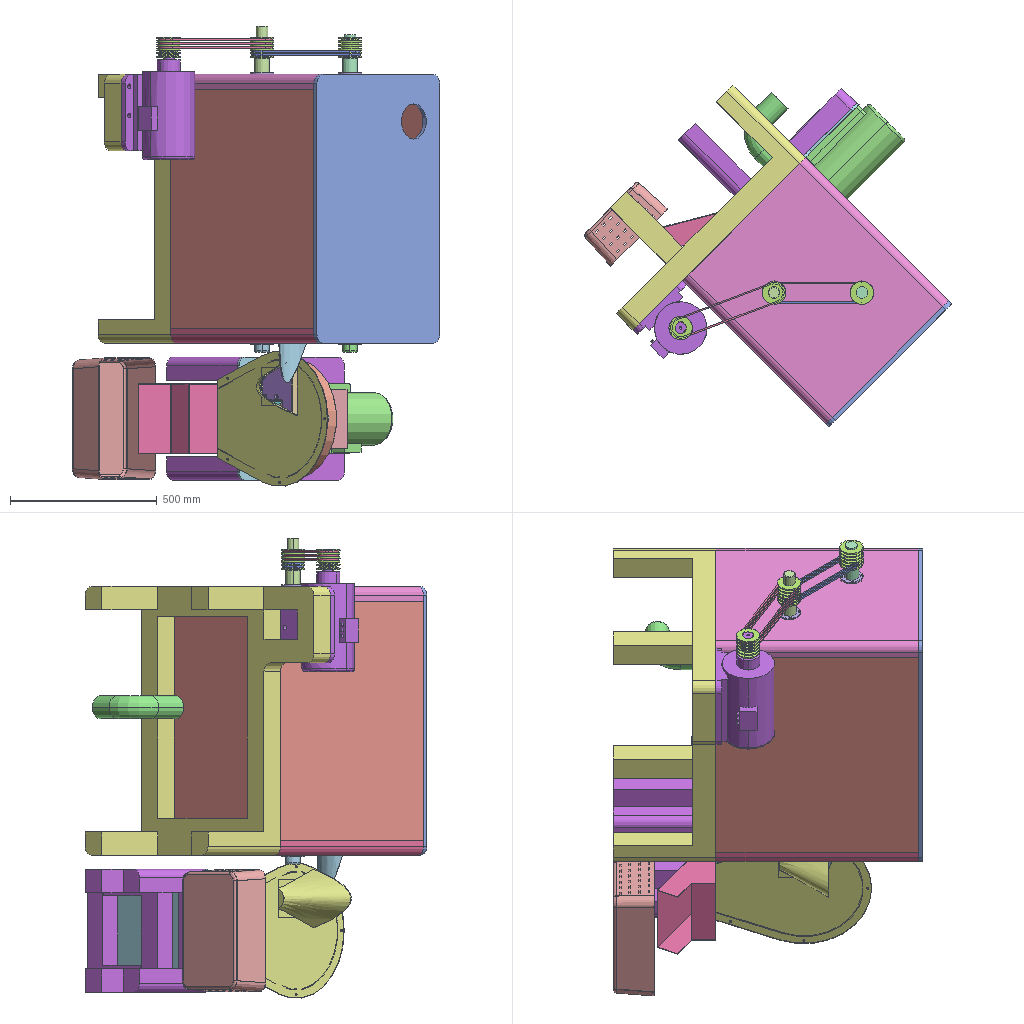Assembly | SolidWorks | 462 different items | 999 placed | box 1253 x 1165 x 1569 mm
Parts list (item | name | quantity | parent item | size | volume | features):
1 | (subassembly) | x1 | in 13 | 390 x 75.007 x 390 mm | 1088681 mm3 | features AEMSimFeature 1
2 | (subassembly) | x1 | in 15 | 456 x 70 x 529.065 mm | 279476 mm3 | features AEMSimFeature 1
3 | (subassembly) | x1 | in 15 | 462 x 531 x 183 mm | 626105 mm3 | features AEMSimFeature 1
4 | (subassembly) | x1 | in 6 | 462 x 872.289 x 730.81 mm | 20879120 mm3 | features AEMSimFeature 1
5 | (subassembly) | x1 | - | 839.689 x 835.894 x 1384 mm | 47233024 mm3 | features AEMSimFeature 1
6 | (subassembly) | x1 | - | - | 106824428 mm3 | features AEMSimFeature 1
7 | (subassembly) | x2 | in 6 | 787.42 x 340 x 340 mm | 9693964 mm3 | features AEMSimFeature 1
8 | (subassembly) | x4 | in 6 | 68 x 19 x 68 mm | 29174 mm3 | features AEMSimFeature 1
9 | (subassembly) | x4 | in 10 | 68 x 68 x 19 mm | 27865 mm3 | features AEMSimFeature 1
10 | (subassembly) | x4 | in 8 | 68 x 19 x 68 mm | 29174 mm3 | features AEMSimFeature 1
11 | (subassembly) | x1 | in 15 | 14 x 62 x 62 mm | 20908 mm3 | features AEMSimFeature 1
12 | (subassembly) | x1 | in 15 | 14 x 62 x 62 mm | 20908 mm3 | features AEMSimFeature 1
13 | (subassembly) | x1 | in 15 | 390 x 210.007 x 390 mm | 3767306 mm3 | features AEMSimFeature 1
14 | (subassembly) | x1 | in 16 | 462 x 451 x 532.065 mm | 5080659 mm3 | features AEMSimFeature 1
15 | (subassembly) | x1 | in 14 | 462 x 532.065 x 451 mm | 5080659 mm3 | features AEMSimFeature 1
16 | (subassembly) | x1 | in 4 | 462 x 451 x 532.065 mm | 5080659 mm3 | features AEMSimFeature 1
17 | (subassembly) | x1 | in 1 | 72 x 14 x 72 mm | 4934 mm3 | features AEMSimFeature 1
18 | - | x2 | in 7 | 10 x 10 x 120 mm | 9425 mm3 | -
19 | - | x2 | in 7 | 10 x 78.624 x 102.96 mm | 9425 mm3 | -
20 | - | x2 | in 7 | 10 x 78.624 x 102.96 mm | 9425 mm3 | -
21 | - | x2 | in 7 | 10 x 102.96 x 78.624 mm | 9425 mm3 | -
22 | - | x2 | in 7 | 10 x 78.624 x 102.96 mm | 9425 mm3 | -
23 | - | x2 | in 7 | 10 x 46.593 x 117.217 mm | 9425 mm3 | -
24 | - | x2 | in 7 | 10 x 102.96 x 78.624 mm | 9425 mm3 | -
25 | - | x2 | in 7 | 10 x 78.624 x 102.96 mm | 9425 mm3 | -
26 | - | x2 | in 7 | 10 x 102.96 x 78.624 mm | 9425 mm3 | -
27 | - | x2 | in 7 | 10 x 46.593 x 117.217 mm | 9425 mm3 | -
28 | - | x2 | in 7 | 10 x 78.624 x 102.96 mm | 9425 mm3 | -
29 | - | x2 | in 7 | 10 x 10 x 120 mm | 9425 mm3 | -
30 | - | x2 | in 7 | 10 x 10 x 120 mm | 9425 mm3 | -
31 | - | x2 | in 7 | 10 x 46.593 x 117.217 mm | 9425 mm3 | -
32 | - | x2 | in 7 | 10 x 10 x 120 mm | 9425 mm3 | -
33 | - | x2 | in 7 | 10 x 78.624 x 102.96 mm | 9425 mm3 | -
34 | - | x2 | in 7 | 10 x 102.96 x 78.624 mm | 9425 mm3 | -
35 | - | x2 | in 7 | 10 x 120 x 10 mm | 9425 mm3 | -
36 | - | x2 | in 7 | 10 x 10 x 120 mm | 9425 mm3 | -
37 | - | x2 | in 7 | 10 x 10 x 120 mm | 9425 mm3 | -
38 | - | x2 | in 7 | 10 x 102.96 x 78.624 mm | 9425 mm3 | -
39 | - | x2 | in 7 | 10 x 120 x 10 mm | 9425 mm3 | -
40 | - | x2 | in 7 | 10 x 78.624 x 102.96 mm | 9425 mm3 | -
41 | - | x2 | in 7 | 10 x 117.217 x 46.593 mm | 9425 mm3 | -
42 | - | x2 | in 7 | 10 x 102.96 x 78.624 mm | 9425 mm3 | -
43 | - | x2 | in 7 | 10 x 117.217 x 46.593 mm | 9425 mm3 | -
44 | - | x2 | in 7 | 10 x 78.624 x 102.96 mm | 9425 mm3 | -
45 | - | x2 | in 7 | 10 x 78.624 x 102.96 mm | 9425 mm3 | -
46 | - | x2 | in 7 | 10 x 117.217 x 46.593 mm | 9425 mm3 | -
47 | - | x2 | in 7 | 10 x 117.217 x 46.593 mm | 9425 mm3 | -
48 | - | x2 | in 7 | 10 x 46.593 x 117.217 mm | 9425 mm3 | -
49 | - | x2 | in 7 | 10 x 46.593 x 117.217 mm | 9425 mm3 | -
50 | - | x2 | in 7 | 10 x 117.217 x 46.593 mm | 9425 mm3 | -
51 | - | x2 | in 7 | 10 x 46.593 x 117.217 mm | 9425 mm3 | -
52 | - | x2 | in 7 | 10 x 102.96 x 78.624 mm | 9425 mm3 | -
53 | - | x2 | in 7 | 10 x 10 x 120 mm | 9425 mm3 | -
54 | - | x2 | in 7 | 10 x 117.217 x 46.593 mm | 9425 mm3 | -
55 | - | x2 | in 7 | 10 x 117.217 x 46.593 mm | 9425 mm3 | -
56 | - | x2 | in 7 | 10 x 46.593 x 117.217 mm | 9425 mm3 | -
57 | - | x2 | in 7 | 10 x 46.593 x 117.217 mm | 9425 mm3 | -
58 | - | x2 | in 7 | 10 x 102.96 x 78.624 mm | 9425 mm3 | -
59 | - | x2 | in 7 | 10 x 102.96 x 78.624 mm | 9425 mm3 | -
60 | - | x2 | in 7 | 10 x 78.624 x 102.96 mm | 9425 mm3 | -
61 | - | x2 | in 7 | 10 x 120 x 10 mm | 9425 mm3 | -
62 | - | x2 | in 7 | 10 x 46.593 x 117.217 mm | 9425 mm3 | -
63 | - | x2 | in 7 | 10 x 117.217 x 46.593 mm | 9425 mm3 | -
64 | - | x2 | in 7 | 10 x 120 x 10 mm | 9425 mm3 | -
65 | - | x2 | in 7 | 10 x 78.624 x 102.96 mm | 9425 mm3 | -
66 | - | x2 | in 7 | 10 x 10 x 120 mm | 9425 mm3 | -
67 | - | x2 | in 7 | 10 x 120 x 10 mm | 9425 mm3 | -
68 | - | x2 | in 7 | 10 x 117.217 x 46.593 mm | 9425 mm3 | -
69 | - | x2 | in 7 | 10 x 117.217 x 46.593 mm | 9425 mm3 | -
70 | - | x2 | in 7 | 10 x 120 x 10 mm | 9425 mm3 | -
71 | - | x2 | in 7 | 10 x 117.217 x 46.593 mm | 9425 mm3 | -
72 | - | x2 | in 7 | 10 x 117.217 x 46.593 mm | 9425 mm3 | -
73 | - | x2 | in 7 | 10 x 10 x 120 mm | 9425 mm3 | -
74 | - | x2 | in 7 | 10 x 78.624 x 102.96 mm | 9425 mm3 | -
75 | - | x2 | in 7 | 10 x 120 x 10 mm | 9425 mm3 | -
76 | - | x2 | in 7 | 10 x 102.96 x 78.624 mm | 9425 mm3 | -
77 | - | x2 | in 7 | 10 x 46.593 x 117.217 mm | 9425 mm3 | -
78 | - | x2 | in 7 | 10 x 120 x 10 mm | 9425 mm3 | -
79 | - | x2 | in 7 | 10 x 102.96 x 78.624 mm | 9425 mm3 | -
80 | - | x2 | in 7 | 10 x 117.217 x 46.593 mm | 9425 mm3 | -
81 | - | x2 | in 7 | 10 x 117.217 x 46.593 mm | 9425 mm3 | -
82 | - | x2 | in 7 | 10 x 46.593 x 117.217 mm | 9425 mm3 | -
83 | - | x2 | in 7 | 10 x 120 x 10 mm | 9425 mm3 | -
84 | - | x2 | in 7 | 10 x 117.217 x 46.593 mm | 9425 mm3 | -
85 | - | x2 | in 7 | 10 x 117.217 x 46.593 mm | 9425 mm3 | -
86 | - | x2 | in 7 | 10 x 78.624 x 102.96 mm | 9425 mm3 | -
87 | - | x2 | in 7 | 10 x 46.593 x 117.217 mm | 9425 mm3 | -
88 | - | x2 | in 7 | 10 x 46.593 x 117.217 mm | 9425 mm3 | -
89 | - | x2 | in 7 | 10 x 10 x 120 mm | 9425 mm3 | -
90 | - | x2 | in 7 | 10 x 78.624 x 102.96 mm | 9425 mm3 | -
91 | - | x2 | in 7 | 10 x 78.624 x 102.96 mm | 9425 mm3 | -
92 | - | x2 | in 7 | 10 x 102.96 x 78.624 mm | 9425 mm3 | -
93 | - | x2 | in 7 | 10 x 102.96 x 78.624 mm | 9425 mm3 | -
94 | - | x2 | in 7 | 10 x 120 x 10 mm | 9425 mm3 | -
95 | - | x2 | in 7 | 10 x 102.96 x 78.624 mm | 9425 mm3 | -
96 | - | x2 | in 7 | 10 x 78.624 x 102.96 mm | 9425 mm3 | -
97 | - | x2 | in 7 | 10 x 102.96 x 78.624 mm | 9425 mm3 | -
98 | - | x2 | in 7 | 10 x 102.96 x 78.624 mm | 9425 mm3 | -
99 | - | x2 | in 7 | 10 x 117.217 x 46.593 mm | 9425 mm3 | -
100 | - | x2 | in 7 | 10 x 10 x 120 mm | 9425 mm3 | -
101 | - | x2 | in 7 | 10 x 117.217 x 46.593 mm | 9425 mm3 | -
102 | - | x2 | in 7 | 10 x 78.624 x 102.96 mm | 9425 mm3 | -
103 | - | x2 | in 7 | 10 x 78.624 x 102.96 mm | 9425 mm3 | -
104 | - | x2 | in 7 | 10 x 10 x 120 mm | 9425 mm3 | -
105 | - | x2 | in 7 | 10 x 117.217 x 46.593 mm | 9425 mm3 | -
106 | - | x2 | in 7 | 10 x 46.593 x 117.217 mm | 9425 mm3 | -
107 | - | x2 | in 7 | 10 x 46.593 x 117.217 mm | 9425 mm3 | -
108 | - | x2 | in 7 | 10 x 102.96 x 78.624 mm | 9425 mm3 | -
109 | - | x2 | in 7 | 10 x 10 x 120 mm | 9425 mm3 | -
110 | - | x2 | in 7 | 10 x 78.624 x 102.96 mm | 9425 mm3 | -
111 | - | x2 | in 7 | 10 x 102.96 x 78.624 mm | 9425 mm3 | -
112 | - | x2 | in 7 | 10 x 46.593 x 117.217 mm | 9425 mm3 | -
113 | - | x2 | in 7 | 10 x 78.624 x 102.96 mm | 9425 mm3 | -
114 | - | x2 | in 7 | 10 x 46.593 x 117.217 mm | 9425 mm3 | -
115 | - | x2 | in 7 | 10 x 46.593 x 117.217 mm | 9425 mm3 | -
116 | - | x2 | in 7 | 10 x 102.96 x 78.624 mm | 9425 mm3 | -
117 | - | x2 | in 7 | 10 x 117.217 x 46.593 mm | 9425 mm3 | -
118 | - | x2 | in 7 | 10 x 78.624 x 102.96 mm | 9425 mm3 | -
119 | - | x2 | in 7 | 10 x 117.217 x 46.593 mm | 9425 mm3 | -
120 | - | x2 | in 7 | 10 x 78.624 x 102.96 mm | 9425 mm3 | -
121 | - | x2 | in 7 | 10 x 120 x 10 mm | 9425 mm3 | -
122 | - | x2 | in 7 | 10 x 78.624 x 102.96 mm | 9425 mm3 | -
123 | - | x2 | in 7 | 10 x 10 x 120 mm | 9425 mm3 | -
124 | - | x2 | in 7 | 10 x 117.217 x 46.593 mm | 9425 mm3 | -
125 | - | x2 | in 7 | 10 x 102.96 x 78.624 mm | 9425 mm3 | -
126 | - | x2 | in 7 | 10 x 102.96 x 78.624 mm | 9425 mm3 | -
127 | - | x2 | in 7 | 10 x 46.593 x 117.217 mm | 9425 mm3 | -
128 | - | x4 | in 9 | 49 x 49 x 19 mm | 11442 mm3 | -
129 | - | x2 | in 7 | 10 x 46.593 x 117.217 mm | 9425 mm3 | -
130 | - | x2 | in 7 | 10 x 102.96 x 78.624 mm | 9425 mm3 | -
131 | - | x2 | in 7 | 10 x 120 x 10 mm | 9425 mm3 | -
132 | - | x2 | in 7 | 10 x 46.593 x 117.217 mm | 9425 mm3 | -
133 | - | x2 | in 7 | 10 x 46.593 x 117.217 mm | 9425 mm3 | -
134 | - | x2 | in 7 | 10 x 46.593 x 117.217 mm | 9425 mm3 | -
135 | - | x2 | in 7 | 10 x 46.593 x 117.217 mm | 9425 mm3 | -
136 | - | x2 | in 7 | 10 x 102.96 x 78.624 mm | 9425 mm3 | -
137 | - | x2 | in 7 | 10 x 102.96 x 78.624 mm | 9425 mm3 | -
138 | - | x2 | in 7 | 10 x 46.593 x 117.217 mm | 9425 mm3 | -
139 | - | x2 | in 7 | 10 x 102.96 x 78.624 mm | 9425 mm3 | -
140 | - | x2 | in 7 | 10 x 102.96 x 78.624 mm | 9425 mm3 | -
141 | - | x2 | in 7 | 10 x 78.624 x 102.96 mm | 9425 mm3 | -
142 | - | x2 | in 7 | 10 x 78.624 x 102.96 mm | 9425 mm3 | -
143 | - | x2 | in 7 | 10 x 46.593 x 117.217 mm | 9425 mm3 | -
144 | - | x2 | in 7 | 10 x 78.624 x 102.96 mm | 9425 mm3 | -
145 | - | x2 | in 7 | 10 x 117.217 x 46.593 mm | 9425 mm3 | -
146 | - | x2 | in 7 | 10 x 78.624 x 102.96 mm | 9425 mm3 | -
147 | - | x2 | in 7 | 10 x 117.217 x 46.593 mm | 9425 mm3 | -
148 | - | x2 | in 7 | 10 x 46.593 x 117.217 mm | 9425 mm3 | -
149 | - | x2 | in 7 | 10 x 46.593 x 117.217 mm | 9425 mm3 | -
150 | - | x2 | in 7 | 10 x 117.217 x 46.593 mm | 9425 mm3 | -
151 | - | x2 | in 7 | 10 x 78.624 x 102.96 mm | 9425 mm3 | -
152 | - | x2 | in 7 | 10 x 10 x 120 mm | 9425 mm3 | -
153 | - | x2 | in 7 | 10 x 46.593 x 117.217 mm | 9425 mm3 | -
154 | - | x2 | in 7 | 10 x 78.624 x 102.96 mm | 9425 mm3 | -
155 | - | x2 | in 7 | 10 x 78.624 x 102.96 mm | 9425 mm3 | -
156 | - | x2 | in 7 | 10 x 102.96 x 78.624 mm | 9425 mm3 | -
157 | - | x2 | in 7 | 10 x 78.624 x 102.96 mm | 9425 mm3 | -
158 | - | x2 | in 7 | 10 x 102.96 x 78.624 mm | 9425 mm3 | -
159 | - | x2 | in 7 | 10 x 46.593 x 117.217 mm | 9425 mm3 | -
160 | - | x2 | in 7 | 10 x 102.96 x 78.624 mm | 9425 mm3 | -
161 | - | x2 | in 7 | 10 x 102.96 x 78.624 mm | 9425 mm3 | -
162 | - | x2 | in 7 | 10 x 117.217 x 46.593 mm | 9425 mm3 | -
163 | - | x2 | in 7 | 10 x 10 x 120 mm | 9425 mm3 | -
164 | - | x2 | in 7 | 10 x 46.593 x 117.217 mm | 9425 mm3 | -
165 | - | x2 | in 7 | 10 x 78.624 x 102.96 mm | 9425 mm3 | -
166 | - | x2 | in 7 | 10 x 117.217 x 46.593 mm | 9425 mm3 | -
167 | - | x2 | in 7 | 10 x 117.217 x 46.593 mm | 9425 mm3 | -
168 | - | x2 | in 7 | 10 x 46.593 x 117.217 mm | 9425 mm3 | -
169 | - | x2 | in 7 | 10 x 78.624 x 102.96 mm | 9425 mm3 | -
170 | - | x2 | in 7 | 10 x 46.593 x 117.217 mm | 9425 mm3 | -
171 | - | x2 | in 7 | 10 x 117.217 x 46.593 mm | 9425 mm3 | -
172 | - | x2 | in 7 | 10 x 117.217 x 46.593 mm | 9425 mm3 | -
173 | - | x2 | in 7 | 10 x 78.624 x 102.96 mm | 9425 mm3 | -
174 | - | x2 | in 7 | 10 x 46.593 x 117.217 mm | 9425 mm3 | -
175 | - | x2 | in 7 | 10 x 120 x 10 mm | 9425 mm3 | -
176 | - | x2 | in 7 | 10 x 78.624 x 102.96 mm | 9425 mm3 | -
177 | - | x2 | in 7 | 10 x 102.96 x 78.624 mm | 9425 mm3 | -
178 | - | x2 | in 7 | 10 x 78.624 x 102.96 mm | 9425 mm3 | -
179 | - | x2 | in 7 | 10 x 120 x 10 mm | 9425 mm3 | -
180 | - | x2 | in 7 | 10 x 102.96 x 78.624 mm | 9425 mm3 | -
181 | - | x2 | in 7 | 10 x 117.217 x 46.593 mm | 9425 mm3 | -
182 | - | x2 | in 7 | 10 x 117.217 x 46.593 mm | 9425 mm3 | -
183 | - | x2 | in 7 | 10 x 120 x 10 mm | 9425 mm3 | -
184 | - | x2 | in 7 | 10 x 102.96 x 78.624 mm | 9425 mm3 | -
185 | - | x2 | in 7 | 10 x 102.96 x 78.624 mm | 9425 mm3 | -
186 | - | x2 | in 7 | 10 x 78.624 x 102.96 mm | 9425 mm3 | -
187 | - | x2 | in 7 | 10 x 120 x 10 mm | 9425 mm3 | -
188 | - | x2 | in 7 | 10 x 117.217 x 46.593 mm | 9425 mm3 | -
189 | - | x2 | in 7 | 10 x 117.217 x 46.593 mm | 9425 mm3 | -
190 | - | x2 | in 7 | 10 x 46.593 x 117.217 mm | 9425 mm3 | -
191 | - | x2 | in 7 | 10 x 78.624 x 102.96 mm | 9425 mm3 | -
192 | - | x2 | in 7 | 10 x 102.96 x 78.624 mm | 9425 mm3 | -
193 | - | x2 | in 7 | 10 x 102.96 x 78.624 mm | 9425 mm3 | -
194 | - | x2 | in 7 | 10 x 46.593 x 117.217 mm | 9425 mm3 | -
195 | - | x2 | in 7 | 10 x 117.217 x 46.593 mm | 9425 mm3 | -
196 | - | x2 | in 7 | 10 x 78.624 x 102.96 mm | 9425 mm3 | -
197 | - | x2 | in 7 | 10 x 120 x 10 mm | 9425 mm3 | -
198 | - | x2 | in 7 | 10 x 117.217 x 46.593 mm | 9425 mm3 | -
199 | - | x2 | in 7 | 10 x 78.624 x 102.96 mm | 9425 mm3 | -
200 | - | x2 | in 7 | 10 x 46.593 x 117.217 mm | 9425 mm3 | -
201 | - | x2 | in 7 | 10 x 46.593 x 117.217 mm | 9425 mm3 | -
202 | - | x2 | in 7 | 10 x 10 x 120 mm | 9425 mm3 | -
203 | - | x2 | in 7 | 10 x 46.593 x 117.217 mm | 9425 mm3 | -
204 | - | x2 | in 7 | 10 x 102.96 x 78.624 mm | 9425 mm3 | -
205 | - | x2 | in 7 | 10 x 78.624 x 102.96 mm | 9425 mm3 | -
206 | - | x2 | in 7 | 10 x 102.96 x 78.624 mm | 9425 mm3 | -
207 | - | x2 | in 7 | 10 x 78.624 x 102.96 mm | 9425 mm3 | -
208 | - | x2 | in 7 | 10 x 46.593 x 117.217 mm | 9425 mm3 | -
209 | - | x2 | in 7 | 10 x 78.624 x 102.96 mm | 9425 mm3 | -
210 | - | x2 | in 7 | 10 x 46.593 x 117.217 mm | 9425 mm3 | -
211 | - | x2 | in 7 | 10 x 78.624 x 102.96 mm | 9425 mm3 | -
212 | - | x2 | in 7 | 10 x 46.593 x 117.217 mm | 9425 mm3 | -
213 | - | x2 | in 7 | 10 x 10 x 120 mm | 9425 mm3 | -
214 | - | x2 | in 7 | 10 x 117.217 x 46.593 mm | 9425 mm3 | -
215 | - | x2 | in 7 | 10 x 78.624 x 102.96 mm | 9425 mm3 | -
216 | - | x2 | in 7 | 10 x 117.217 x 46.593 mm | 9425 mm3 | -
217 | - | x2 | in 7 | 10 x 10 x 120 mm | 9425 mm3 | -
218 | - | x2 | in 7 | 10 x 117.217 x 46.593 mm | 9425 mm3 | -
219 | - | x2 | in 7 | 10 x 120 x 10 mm | 9425 mm3 | -
220 | - | x2 | in 7 | 10 x 46.593 x 117.217 mm | 9425 mm3 | -
221 | - | x2 | in 7 | 10 x 46.593 x 117.217 mm | 9425 mm3 | -
222 | - | x2 | in 7 | 10 x 117.217 x 46.593 mm | 9425 mm3 | -
223 | - | x2 | in 7 | 10 x 120 x 10 mm | 9425 mm3 | -
224 | - | x2 | in 7 | 10 x 78.624 x 102.96 mm | 9425 mm3 | -
225 | - | x2 | in 7 | 10 x 78.624 x 102.96 mm | 9425 mm3 | -
226 | - | x2 | in 7 | 10 x 46.593 x 117.217 mm | 9425 mm3 | -
227 | - | x2 | in 7 | 10 x 46.593 x 117.217 mm | 9425 mm3 | -
228 | - | x2 | in 7 | 10 x 10 x 120 mm | 9425 mm3 | -
229 | - | x2 | in 7 | 10 x 10 x 120 mm | 9425 mm3 | -
230 | - | x2 | in 7 | 10 x 10 x 120 mm | 9425 mm3 | -
231 | - | x2 | in 7 | 10 x 46.593 x 117.217 mm | 9425 mm3 | -
232 | - | x2 | in 7 | 10 x 102.96 x 78.624 mm | 9425 mm3 | -
233 | - | x2 | in 7 | 10 x 46.593 x 117.217 mm | 9425 mm3 | -
234 | - | x2 | in 7 | 10 x 117.217 x 46.593 mm | 9425 mm3 | -
235 | - | x2 | in 7 | 10 x 120 x 10 mm | 9425 mm3 | -
236 | - | x2 | in 7 | 10 x 117.217 x 46.593 mm | 9425 mm3 | -
237 | - | x2 | in 7 | 10 x 117.217 x 46.593 mm | 9425 mm3 | -
238 | - | x2 | in 7 | 10 x 117.217 x 46.593 mm | 9425 mm3 | -
239 | - | x4 | in 9 | 68 x 68 x 19 mm | 16423 mm3 | -
240 | - | x2 | in 7 | 10 x 78.624 x 102.96 mm | 9425 mm3 | -
241 | - | x2 | in 7 | 10 x 78.624 x 102.96 mm | 9425 mm3 | -
242 | - | x2 | in 7 | 10 x 120 x 10 mm | 9425 mm3 | -
243 | - | x2 | in 7 | 10 x 78.624 x 102.96 mm | 9425 mm3 | -
244 | - | x2 | in 7 | 10 x 78.624 x 102.96 mm | 9425 mm3 | -
245 | - | x2 | in 7 | 10 x 102.96 x 78.624 mm | 9425 mm3 | -
246 | - | x2 | in 7 | 10 x 102.96 x 78.624 mm | 9425 mm3 | -
247 | - | x2 | in 7 | 10 x 46.593 x 117.217 mm | 9425 mm3 | -
248 | - | x2 | in 7 | 10 x 78.624 x 102.96 mm | 9425 mm3 | -
249 | - | x2 | in 7 | 10 x 120 x 10 mm | 9425 mm3 | -
250 | - | x2 | in 7 | 10 x 102.96 x 78.624 mm | 9425 mm3 | -
251 | - | x2 | in 7 | 10 x 10 x 120 mm | 9425 mm3 | -
252 | - | x2 | in 7 | 10 x 102.96 x 78.624 mm | 9425 mm3 | -
253 | - | x2 | in 7 | 10 x 120 x 10 mm | 9425 mm3 | -
254 | - | x2 | in 7 | 10 x 120 x 10 mm | 9425 mm3 | -
255 | - | x2 | in 7 | 10 x 46.593 x 117.217 mm | 9425 mm3 | -
256 | - | x2 | in 7 | 10 x 10 x 120 mm | 9425 mm3 | -
257 | - | x2 | in 7 | 10 x 10 x 120 mm | 9425 mm3 | -
258 | - | x2 | in 7 | 10 x 46.593 x 117.217 mm | 9425 mm3 | -
259 | - | x2 | in 7 | 10 x 102.96 x 78.624 mm | 9425 mm3 | -
260 | - | x2 | in 7 | 10 x 10 x 120 mm | 9425 mm3 | -
261 | - | x2 | in 7 | 10 x 120 x 10 mm | 9425 mm3 | -
262 | - | x2 | in 7 | 10 x 120 x 10 mm | 9425 mm3 | -
263 | - | x2 | in 7 | 10 x 117.217 x 46.593 mm | 9425 mm3 | -
264 | - | x2 | in 7 | 10 x 117.217 x 46.593 mm | 9425 mm3 | -
265 | - | x2 | in 7 | 10 x 46.593 x 117.217 mm | 9425 mm3 | -
266 | - | x2 | in 7 | 10 x 46.593 x 117.217 mm | 9425 mm3 | -
267 | - | x2 | in 7 | 10 x 117.217 x 46.593 mm | 9425 mm3 | -
268 | - | x2 | in 7 | 10 x 117.217 x 46.593 mm | 9425 mm3 | -
269 | - | x2 | in 7 | 10 x 102.96 x 78.624 mm | 9425 mm3 | -
270 | - | x2 | in 7 | 10 x 46.593 x 117.217 mm | 9425 mm3 | -
271 | - | x2 | in 7 | 10 x 102.96 x 78.624 mm | 9425 mm3 | -
272 | - | x2 | in 7 | 10 x 10 x 120 mm | 9425 mm3 | -
273 | - | x2 | in 7 | 10 x 120 x 10 mm | 9425 mm3 | -
274 | - | x2 | in 7 | 10 x 78.624 x 102.96 mm | 9425 mm3 | -
275 | - | x2 | in 7 | 10 x 10 x 120 mm | 9425 mm3 | -
276 | - | x2 | in 7 | 10 x 10 x 120 mm | 9425 mm3 | -
277 | - | x2 | in 7 | 10 x 102.96 x 78.624 mm | 9425 mm3 | -
278 | - | x2 | in 7 | 10 x 78.624 x 102.96 mm | 9425 mm3 | -
279 | - | x2 | in 7 | 10 x 102.96 x 78.624 mm | 9425 mm3 | -
280 | - | x2 | in 7 | 10 x 78.624 x 102.96 mm | 9425 mm3 | -
281 | - | x2 | in 7 | 10 x 117.217 x 46.593 mm | 9425 mm3 | -
282 | - | x2 | in 7 | 10 x 78.624 x 102.96 mm | 9425 mm3 | -
283 | - | x2 | in 7 | 10 x 120 x 10 mm | 9425 mm3 | -
284 | - | x2 | in 7 | 10 x 102.96 x 78.624 mm | 9425 mm3 | -
285 | - | x2 | in 7 | 10 x 102.96 x 78.624 mm | 9425 mm3 | -
286 | - | x2 | in 7 | 10 x 78.624 x 102.96 mm | 9425 mm3 | -
287 | - | x2 | in 7 | 10 x 102.96 x 78.624 mm | 9425 mm3 | -
288 | - | x2 | in 7 | 10 x 102.96 x 78.624 mm | 9425 mm3 | -
289 | - | x2 | in 7 | 10 x 102.96 x 78.624 mm | 9425 mm3 | -
290 | - | x2 | in 7 | 10 x 120 x 10 mm | 9425 mm3 | -
291 | - | x2 | in 7 | 10 x 120 x 10 mm | 9425 mm3 | -
292 | - | x2 | in 7 | 10 x 46.593 x 117.217 mm | 9425 mm3 | -
293 | - | x2 | in 7 | 10 x 78.624 x 102.96 mm | 9425 mm3 | -
294 | - | x2 | in 7 | 10 x 78.624 x 102.96 mm | 9425 mm3 | -
295 | - | x2 | in 7 | 10 x 102.96 x 78.624 mm | 9425 mm3 | -
296 | - | x2 | in 7 | 10 x 10 x 120 mm | 9425 mm3 | -
297 | - | x2 | in 7 | 10 x 102.96 x 78.624 mm | 9425 mm3 | -
298 | - | x2 | in 7 | 10 x 46.593 x 117.217 mm | 9425 mm3 | -
299 | - | x2 | in 7 | 10 x 46.593 x 117.217 mm | 9425 mm3 | -
300 | - | x2 | in 7 | 10 x 117.217 x 46.593 mm | 9425 mm3 | -
301 | - | x2 | in 7 | 10 x 10 x 120 mm | 9425 mm3 | -
302 | - | x2 | in 7 | 10 x 102.96 x 78.624 mm | 9425 mm3 | -
303 | - | x2 | in 7 | 10 x 46.593 x 117.217 mm | 9425 mm3 | -
304 | - | x2 | in 7 | 10 x 117.217 x 46.593 mm | 9425 mm3 | -
305 | - | x2 | in 7 | 10 x 102.96 x 78.624 mm | 9425 mm3 | -
306 | - | x2 | in 7 | 10 x 46.593 x 117.217 mm | 9425 mm3 | -
307 | - | x2 | in 7 | 10 x 120 x 10 mm | 9425 mm3 | -
308 | - | x2 | in 7 | 10 x 117.217 x 46.593 mm | 9425 mm3 | -
309 | - | x2 | in 7 | 10 x 102.96 x 78.624 mm | 9425 mm3 | -
310 | - | x2 | in 7 | 10 x 78.624 x 102.96 mm | 9425 mm3 | -
311 | - | x2 | in 7 | 10 x 120 x 10 mm | 9425 mm3 | -
312 | - | x2 | in 7 | 10 x 117.217 x 46.593 mm | 9425 mm3 | -
313 | - | x2 | in 7 | 10 x 78.624 x 102.96 mm | 9425 mm3 | -
314 | - | x2 | in 7 | 10 x 78.624 x 102.96 mm | 9425 mm3 | -
315 | - | x2 | in 7 | 10 x 46.593 x 117.217 mm | 9425 mm3 | -
316 | - | x2 | in 7 | 10 x 46.593 x 117.217 mm | 9425 mm3 | -
317 | - | x2 | in 7 | 10 x 117.217 x 46.593 mm | 9425 mm3 | -
318 | - | x2 | in 7 | 10 x 102.96 x 78.624 mm | 9425 mm3 | -
319 | - | x2 | in 7 | 10 x 78.624 x 102.96 mm | 9425 mm3 | -
320 | - | x2 | in 7 | 10 x 78.624 x 102.96 mm | 9425 mm3 | -
321 | - | x2 | in 7 | 10 x 102.96 x 78.624 mm | 9425 mm3 | -
322 | - | x2 | in 7 | 10 x 102.96 x 78.624 mm | 9425 mm3 | -
323 | - | x2 | in 7 | 10 x 102.96 x 78.624 mm | 9425 mm3 | -
324 | - | x2 | in 7 | 10 x 46.593 x 117.217 mm | 9425 mm3 | -
325 | - | x2 | in 7 | 10 x 117.217 x 46.593 mm | 9425 mm3 | -
326 | - | x2 | in 7 | 10 x 46.593 x 117.217 mm | 9425 mm3 | -
327 | - | x2 | in 7 | 10 x 78.624 x 102.96 mm | 9425 mm3 | -
328 | - | x2 | in 7 | 10 x 46.593 x 117.217 mm | 9425 mm3 | -
329 | - | x2 | in 7 | 10 x 46.593 x 117.217 mm | 9425 mm3 | -
330 | - | x2 | in 7 | 10 x 117.217 x 46.593 mm | 9425 mm3 | -
331 | - | x2 | in 7 | 10 x 78.624 x 102.96 mm | 9425 mm3 | -
332 | - | x2 | in 7 | 10 x 78.624 x 102.96 mm | 9425 mm3 | -
333 | - | x2 | in 7 | 10 x 46.593 x 117.217 mm | 9425 mm3 | -
334 | - | x2 | in 7 | 10 x 117.217 x 46.593 mm | 9425 mm3 | -
335 | - | x2 | in 7 | 10 x 78.624 x 102.96 mm | 9425 mm3 | -
336 | - | x2 | in 7 | 10 x 120 x 10 mm | 9425 mm3 | -
337 | - | x2 | in 7 | 10 x 120 x 10 mm | 9425 mm3 | -
338 | - | x2 | in 7 | 10 x 102.96 x 78.624 mm | 9425 mm3 | -
339 | - | x2 | in 7 | 10 x 102.96 x 78.624 mm | 9425 mm3 | -
340 | - | x2 | in 7 | 10 x 46.593 x 117.217 mm | 9425 mm3 | -
341 | - | x2 | in 7 | 10 x 10 x 120 mm | 9425 mm3 | -
342 | - | x2 | in 7 | 10 x 117.217 x 46.593 mm | 9425 mm3 | -
343 | - | x2 | in 7 | 10 x 46.593 x 117.217 mm | 9425 mm3 | -
344 | - | x2 | in 7 | 10 x 10 x 120 mm | 9425 mm3 | -
345 | - | x2 | in 7 | 10 x 102.96 x 78.624 mm | 9425 mm3 | -
346 | - | x2 | in 7 | 10 x 78.624 x 102.96 mm | 9425 mm3 | -
347 | - | x2 | in 7 | 10 x 102.96 x 78.624 mm | 9425 mm3 | -
348 | - | x2 | in 7 | 10 x 120 x 10 mm | 9425 mm3 | -
349 | - | x2 | in 7 | 10 x 46.593 x 117.217 mm | 9425 mm3 | -
350 | - | x2 | in 7 | 10 x 78.624 x 102.96 mm | 9425 mm3 | -
351 | - | x2 | in 7 | 10 x 120 x 10 mm | 9425 mm3 | -
352 | - | x2 | in 7 | 10 x 117.217 x 46.593 mm | 9425 mm3 | -
353 | - | x2 | in 7 | 10 x 46.593 x 117.217 mm | 9425 mm3 | -
354 | - | x2 | in 7 | 10 x 117.217 x 46.593 mm | 9425 mm3 | -
355 | - | x14 | in 11 | 4.2 x 4.2 x 4.2 mm | 38.792 mm3 | -
356 | - | x14 | in 12 | 4.2 x 4.2 x 4.2 mm | 38.792 mm3 | -
357 | - | x1 | in 11 | 14 x 45.385 x 45.385 mm | 7900 mm3 | -
358 | - | x1 | in 12 | 14 x 45.385 x 45.385 mm | 7900 mm3 | -
359 | - | x1 | in 11 | 14 x 62 x 62 mm | 12465 mm3 | -
360 | - | x1 | in 12 | 14 x 62 x 62 mm | 12465 mm3 | -
361 | - | x1 | in 17 | 72 x 6 x 72 mm | 3619 mm3 | -
362 | - | x2 | in 7 | 10 x 78.624 x 102.96 mm | 9425 mm3 | -
363 | - | x1 | in 17 | 55 x 4 x 55 mm | 1315 mm3 | -
364 | - | x1 | in 15 | 35 x 255 x 35 mm | 172975 mm3 | -
365 | - | x1 | in 15 | 120 x 40 x 120 mm | 192967 mm3 | -
366 | - | x1 | in 4 | 205.061 x 205.061 x 118 mm | 15916 mm3 | -
367 | - | x1 | in 6 | 906.604 x 906.604 x 50 mm | 19871305 mm3 | -
368 | - | x1 | in 4 | 240 x 200 x 417.5 mm | 9698693 mm3 | -
369 | - | x1 | in 13 | 200 x 120 x 200 mm | 2678625 mm3 | -
370 | - | x1 | in 4 | 374.767 x 516.188 x 420 mm | 5744112 mm3 | -
371 | - | x1 | in 4 | 318.967 x 186.877 x 240 mm | 339701 mm3 | -
372 | - | x2 | in 1 | 51.059 x 17.007 x 160 mm | 32939 mm3 | -
373 | - | x2 | in 7 | 10 x 102.96 x 78.624 mm | 9425 mm3 | -
374 | - | x2 | in 1 | 51.059 x 17.007 x 160 mm | 34219 mm3 | -
375 | - | x1 | in 1 | 60 x 70 x 60 mm | 151590 mm3 | -
376 | - | x1 | in 1 | 390 x 8 x 390 mm | 797841 mm3 | -
377 | - | x1 | in 2 | 406 x 70 x 504.065 mm | 266533 mm3 | -
378 | - | x1 | in 2 | - | - | features BaseBody 1
379 | - | x5 | in 2 | 20 x 25 x 25 mm | 2589 mm3 | -
380 | - | x1 | in 3 | 462 x 531 x 183 mm | 626105 mm3 | -
381 | - | x1 | in 6 | 906.604 x 906.604 x 50 mm | 18863747 mm3 | -
382 | - | x1 | in 6 | 94.546 x 86.364 x 182.8 mm | 42412 mm3 | -
383 | - | x1 | in 5 | 606.344 x 425.772 x 420 mm | 17162651 mm3 | -
384 | - | x2 | in 7 | 10 x 117.217 x 46.593 mm | 9425 mm3 | -
385 | - | x4 | in 6 | 80 x 80 x 16 mm | 27390 mm3 | -
386 | - | x4 | in 6 | 80 x 80 x 70 mm | 197004 mm3 | -
387 | - | x1 | - | 176.563 x 311.125 x 80 mm | 356270 mm3 | -
388 | - | x1 | - | 414.674 x 140 x 274.674 mm | 549320 mm3 | features Fillet 2, Extrusion 1, ICE 1, LPattern 1, Shell 1
389 | - | x2 | in 7 | 10 x 102.96 x 78.624 mm | 9425 mm3 | -
390 | - | x2 | in 7 | 10 x 78.624 x 102.96 mm | 9425 mm3 | -
391 | - | x1 | in 6 | 180.002 x 50 x 50 mm | 309551 mm3 | -
392 | - | x1 | - | 429.306 x 429.306 x 917.42 mm | 7967244 mm3 | -
393 | - | x1 | in 5 | 666.188 x 835.894 x 917.42 mm | 30070373 mm3 | -
394 | - | x80 | in 10 | 5 x 5 x 5 mm | 65.45 mm3 | -
395 | - | x2 | in 7 | 10 x 78.624 x 102.96 mm | 9425 mm3 | -
396 | - | x1 | in 6 | 240 x 200 x 417.5 mm | 9686675 mm3 | -
397 | - | x1 | in 6 | 285.002 x 50 x 50 mm | 456683 mm3 | -
398 | - | x3 | in 6 | 388.198 x 190.208 x 7 mm | 30957 mm3 | -
399 | - | x2 | in 6 | 370 x 70 x 7 mm | 28147 mm3 | -
400 | - | x1 | in 6 | 906.604 x 906.604 x 817.42 mm | 15906852 mm3 | -
401 | - | x1 | - | 180.002 x 50 x 50 mm | 309551 mm3 | -
402 | - | x2 | in 7 | 10 x 102.96 x 78.624 mm | 9425 mm3 | -
403 | - | x2 | in 7 | 10 x 117.217 x 46.593 mm | 9425 mm3 | -
404 | - | x2 | in 7 | 10 x 117.217 x 46.593 mm | 9425 mm3 | -
405 | - | x2 | in 7 | 10 x 102.96 x 78.624 mm | 9425 mm3 | -
406 | - | x2 | in 7 | 10 x 10 x 120 mm | 9425 mm3 | -
407 | - | x2 | in 7 | 10 x 10 x 120 mm | 9425 mm3 | -
408 | - | x2 | in 7 | 10 x 117.217 x 46.593 mm | 9425 mm3 | -
409 | - | x2 | in 7 | 10 x 102.96 x 78.624 mm | 9425 mm3 | -
410 | - | x2 | in 7 | 10 x 46.593 x 117.217 mm | 9425 mm3 | -
411 | - | x2 | in 7 | 10 x 46.593 x 117.217 mm | 9425 mm3 | -
412 | - | x2 | in 7 | 10 x 10 x 120 mm | 9425 mm3 | -
413 | - | x2 | in 7 | 10 x 117.217 x 46.593 mm | 9425 mm3 | -
414 | - | x2 | in 7 | 10 x 102.96 x 78.624 mm | 9425 mm3 | -
415 | - | x2 | in 7 | 10 x 120 x 10 mm | 9425 mm3 | -
416 | - | x2 | in 7 | 10 x 120 x 10 mm | 9425 mm3 | -
417 | - | x2 | in 7 | 10 x 46.593 x 117.217 mm | 9425 mm3 | -
418 | - | x2 | in 7 | 10 x 10 x 120 mm | 9425 mm3 | -
419 | - | x2 | in 7 | 10 x 46.593 x 117.217 mm | 9425 mm3 | -
420 | - | x2 | in 7 | 10 x 78.624 x 102.96 mm | 9425 mm3 | -
421 | - | x2 | in 7 | 10 x 117.217 x 46.593 mm | 9425 mm3 | -
422 | - | x2 | in 7 | 10 x 117.217 x 46.593 mm | 9425 mm3 | -
423 | - | x2 | in 7 | 10 x 102.96 x 78.624 mm | 9425 mm3 | -
424 | - | x2 | in 7 | 10 x 117.217 x 46.593 mm | 9425 mm3 | -
425 | - | x2 | in 7 | 10 x 117.217 x 46.593 mm | 9425 mm3 | -
426 | - | x2 | in 7 | 10 x 117.217 x 46.593 mm | 9425 mm3 | -
427 | - | x2 | in 7 | 10 x 10 x 120 mm | 9425 mm3 | -
428 | - | x2 | in 7 | 10 x 117.217 x 46.593 mm | 9425 mm3 | -
429 | - | x2 | in 7 | 10 x 46.593 x 117.217 mm | 9425 mm3 | -
430 | - | x2 | in 7 | 10 x 78.624 x 102.96 mm | 9425 mm3 | -
431 | - | x2 | in 7 | 10 x 120 x 10 mm | 9425 mm3 | -
432 | - | x2 | in 7 | 10 x 117.217 x 46.593 mm | 9425 mm3 | -
433 | - | x2 | in 7 | 10 x 78.624 x 102.96 mm | 9425 mm3 | -
434 | - | x2 | in 7 | 10 x 102.96 x 78.624 mm | 9425 mm3 | -
435 | - | x2 | in 7 | 10 x 46.593 x 117.217 mm | 9425 mm3 | -
436 | - | x2 | in 7 | 10 x 117.217 x 46.593 mm | 9425 mm3 | -
437 | - | x2 | in 7 | 10 x 10 x 120 mm | 9425 mm3 | -
438 | - | x2 | in 7 | 10 x 117.217 x 46.593 mm | 9425 mm3 | -
439 | - | x2 | in 7 | 10 x 117.217 x 46.593 mm | 9425 mm3 | -
440 | - | x2 | in 7 | 10 x 102.96 x 78.624 mm | 9425 mm3 | -
441 | - | x2 | in 7 | 10 x 117.217 x 46.593 mm | 9425 mm3 | -
442 | - | x2 | in 7 | 10 x 78.624 x 102.96 mm | 9425 mm3 | -
443 | - | x2 | in 7 | 10 x 102.96 x 78.624 mm | 9425 mm3 | -
444 | - | x2 | in 7 | 10 x 117.217 x 46.593 mm | 9425 mm3 | -
445 | - | x2 | in 7 | 10 x 102.96 x 78.624 mm | 9425 mm3 | -
446 | - | x2 | in 7 | 10 x 102.96 x 78.624 mm | 9425 mm3 | -
447 | - | x2 | in 7 | 10 x 46.593 x 117.217 mm | 9425 mm3 | -
448 | - | x2 | in 7 | 10 x 46.593 x 117.217 mm | 9425 mm3 | -
449 | - | x2 | in 7 | 787.42 x 100 x 100 mm | 5924053 mm3 | -
450 | - | x2 | in 7 | 10 x 102.96 x 78.624 mm | 9425 mm3 | -
451 | - | x2 | in 7 | 10 x 46.593 x 117.217 mm | 9425 mm3 | -
452 | - | x2 | in 7 | 10 x 117.217 x 46.593 mm | 9425 mm3 | -
453 | - | x2 | in 7 | 10 x 102.96 x 78.624 mm | 9425 mm3 | -
454 | - | x2 | in 7 | 10 x 78.624 x 102.96 mm | 9425 mm3 | -
455 | - | x2 | in 7 | 10 x 117.217 x 46.593 mm | 9425 mm3 | -
456 | - | x2 | in 7 | 10 x 46.593 x 117.217 mm | 9425 mm3 | -
457 | - | x2 | in 7 | 10 x 10 x 120 mm | 9425 mm3 | -
458 | - | x2 | in 7 | 10 x 117.217 x 46.593 mm | 9425 mm3 | -
459 | - | x2 | in 7 | 10 x 78.624 x 102.96 mm | 9425 mm3 | -
460 | - | x2 | in 7 | 10 x 120 x 10 mm | 9425 mm3 | -
461 | - | x2 | in 7 | 10 x 78.624 x 102.96 mm | 9425 mm3 | -
462 | - | x1 | in 6 | 315.002 x 50 x 50 mm | 494133 mm3 | -
Mates (type | each side: item.copy, entity, surface, feature):
Coincident | 388.1 face plane 凸台-拉伸1 | 393.1 face plane Imported1
Width | 388.1 face plane 凸台-拉伸1 | 388.1 face plane 凸台-拉伸1 | 371.1 face plane Imported1 | 371.1 face plane Imported1
DistanceDim | 388.1 edge | 383.1 face plane Imported1